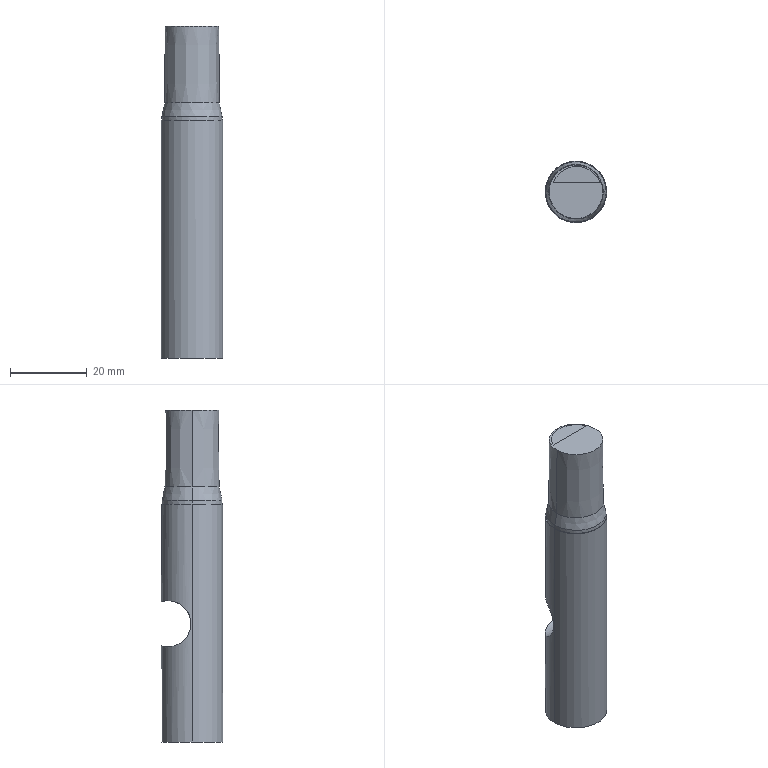Part | Creo | 1 solid | 13 faces | box 16 x 16 x 86.655 mm | volume 15519 mm3 | cylinder 5 | plane 4 | cone 4 | commonest cylinder face diameters 15.678 x2 16 x2 12 x1
STEP:
#1=CARTESIAN_POINT('',(0.,0.,0.));
#2=DIRECTION('',(0.,0.,1.));
#3=DIRECTION('',(1.,0.,0.));
#4=AXIS2_PLACEMENT_3D('',#1,#2,#3);
#5=CARTESIAN_POINT('',(-83.209,27.679,-128.582));
#6=VERTEX_POINT('',#5);
#7=CARTESIAN_POINT('',(-83.208,27.678,-116.581));
#8=VERTEX_POINT('',#7);
#9=CARTESIAN_POINT('',(-83.209,27.679,-128.582));
#10=CARTESIAN_POINT('',(-82.861,27.406,-128.582));
#11=CARTESIAN_POINT('',(-82.24,26.826,-128.543));
#12=CARTESIAN_POINT('',(-81.527,25.921,-128.344));
#13=CARTESIAN_POINT('',(-80.996,25.018,-127.988));
#14=CARTESIAN_POINT('',(-80.628,24.165,-127.48));
#15=CARTESIAN_POINT('',(-80.382,23.365,-126.798));
#16=CARTESIAN_POINT('',(-80.24,22.661,-125.935));
#17=CARTESIAN_POINT('',(-80.176,22.114,-124.925));
#18=CARTESIAN_POINT('',(-80.154,21.761,-123.789));
#19=CARTESIAN_POINT('',(-80.151,21.638,-122.589));
#20=CARTESIAN_POINT('',(-80.154,21.757,-121.388));
#21=CARTESIAN_POINT('',(-80.175,22.112,-120.237));
#22=CARTESIAN_POINT('',(-80.243,22.679,-119.196));
#23=CARTESIAN_POINT('',(-80.392,23.407,-118.321));
#24=CARTESIAN_POINT('',(-80.647,24.216,-117.646));
#25=CARTESIAN_POINT('',(-81.024,25.072,-117.148));
#26=CARTESIAN_POINT('',(-81.554,25.958,-116.808));
#27=CARTESIAN_POINT('',(-82.253,26.838,-116.618));
#28=CARTESIAN_POINT('',(-82.865,27.409,-116.581));
#29=CARTESIAN_POINT('',(-83.208,27.678,-116.581));
#30=B_SPLINE_CURVE_WITH_KNOTS('',3,(#9,#10,#11,#12,#13,#14,#15,#16,#17,#18,#19,#20,#21,#22,#23,#24,#25,#26,#27,#28,#29),.UNSPECIFIED.,.F.,.F.,(4,1,1,1,1,1,1,1,1,1,1,1,1,1,1,1,1,1,4),(0.,0.05556,0.1111,0.1667,0.2222,0.2778,0.3333,0.3889,0.4444,0.5,0.5556,0.6111,0.6667,0.7222,0.7778,0.8333,0.8889,0.9444,1.),.UNSPECIFIED.);
#31=EDGE_CURVE('',#6,#8,#30,.T.);
#32=ORIENTED_EDGE('',*,*,#31,.T.);
#33=CARTESIAN_POINT('',(-93.085,27.679,-116.581));
#34=VERTEX_POINT('',#33);
#35=CARTESIAN_POINT('',(-83.552,27.948,-116.581));
#36=CARTESIAN_POINT('',(-84.287,28.434,-116.617));
#37=CARTESIAN_POINT('',(-85.512,28.978,-116.718));
#38=CARTESIAN_POINT('',(-86.821,29.312,-116.806));
#39=CARTESIAN_POINT('',(-88.163,29.423,-116.84));
#40=CARTESIAN_POINT('',(-89.528,29.305,-116.804));
#41=CARTESIAN_POINT('',(-90.861,28.951,-116.711));
#42=CARTESIAN_POINT('',(-92.076,28.393,-116.612));
#43=CARTESIAN_POINT('',(-92.767,27.928,-116.581));
#44=CARTESIAN_POINT('',(-93.085,27.679,-116.581));
#45=B_SPLINE_CURVE_WITH_KNOTS('',3,(#7,#35,#36,#37,#38,#39,#40,#41,#42,#43,#44),.UNSPECIFIED.,.F.,.F.,(4,1,1,1,1,1,1,1,4),(0.,0.125,0.25,0.375,0.5,0.625,0.75,0.875,1.),.UNSPECIFIED.);
#46=EDGE_CURVE('',#8,#34,#45,.T.);
#47=ORIENTED_EDGE('',*,*,#46,.T.);
#48=CARTESIAN_POINT('',(-93.431,27.407,-116.581));
#49=CARTESIAN_POINT('',(-94.052,26.827,-116.618));
#50=CARTESIAN_POINT('',(-94.78,25.902,-116.823));
#51=CARTESIAN_POINT('',(-95.314,24.985,-117.189));
#52=CARTESIAN_POINT('',(-95.687,24.107,-117.721));
#53=CARTESIAN_POINT('',(-95.928,23.295,-118.435));
#54=CARTESIAN_POINT('',(-96.061,22.605,-119.313));
#55=CARTESIAN_POINT('',(-96.121,22.075,-120.331));
#56=CARTESIAN_POINT('',(-96.139,21.74,-121.477));
#57=CARTESIAN_POINT('',(-96.142,21.639,-122.684));
#58=CARTESIAN_POINT('',(-96.138,21.78,-123.88));
#59=CARTESIAN_POINT('',(-96.114,22.151,-125.013));
#60=CARTESIAN_POINT('',(-96.043,22.725,-126.032));
#61=CARTESIAN_POINT('',(-95.887,23.46,-126.895));
#62=CARTESIAN_POINT('',(-95.613,24.309,-127.584));
#63=CARTESIAN_POINT('',(-95.188,25.231,-128.091));
#64=CARTESIAN_POINT('',(-94.589,26.175,-128.416));
#65=CARTESIAN_POINT('',(-93.793,27.099,-128.576));
#66=CARTESIAN_POINT('',(-92.784,27.951,-128.592));
#67=CARTESIAN_POINT('',(-91.577,28.66,-128.511));
#68=CARTESIAN_POINT('',(-90.18,29.171,-128.397));
#69=CARTESIAN_POINT('',(-88.698,29.411,-128.326));
#70=CARTESIAN_POINT('',(-87.235,29.379,-128.336));
#71=CARTESIAN_POINT('',(-85.753,29.068,-128.424));
#72=CARTESIAN_POINT('',(-84.373,28.489,-128.539));
#73=CARTESIAN_POINT('',(-83.576,27.967,-128.582));
#74=B_SPLINE_CURVE_WITH_KNOTS('',3,(#33,#48,#49,#50,#51,#52,#53,#54,#55,#56,#57,#58,#59,#60,#61,#62,#63,#64,#65,#66,#67,#68,#69,#70,#71,#72,#73,#5),.UNSPECIFIED.,.F.,.F.,(4,1,1,1,1,1,1,1,1,1,1,1,1,1,1,1,1,1,1,1,1,1,1,1,1,4),(0.,0.04,0.08,0.12,0.16,0.2,0.24,0.28,0.32,0.36,0.4,0.44,0.48,0.52,0.56,0.6,0.64,0.68,0.72,0.76,0.8,0.84,0.88,0.92,0.96,1.),.UNSPECIFIED.);
#75=EDGE_CURVE('',#34,#6,#74,.T.);
#76=ORIENTED_EDGE('',*,*,#75,.T.);
#77=EDGE_LOOP('',(#32,#47,#76));
#78=FACE_OUTER_BOUND('',#77,.F.);
#79=CARTESIAN_POINT('',(389.101,27.678,-122.581));
#80=DIRECTION('',(-1.,0.,0.));
#81=DIRECTION('',(0.,0.,1.));
#82=AXIS2_PLACEMENT_3D('',#79,#80,#81);
#83=CYLINDRICAL_SURFACE('',#82,6.);
#84=ADVANCED_FACE('',(#78),#83,.F.);
#85=CARTESIAN_POINT('',(-96.147,21.385,-153.441));
#86=VERTEX_POINT('',#85);
#87=CARTESIAN_POINT('',(-80.147,21.385,-153.441));
#88=VERTEX_POINT('',#87);
#89=CARTESIAN_POINT('',(-88.147,21.385,-153.441));
#90=DIRECTION('',(0.,0.,-1.));
#91=DIRECTION('',(-1.,0.,0.));
#92=AXIS2_PLACEMENT_3D('',#89,#90,#91);
#93=CIRCLE('',#92,8.);
#94=EDGE_CURVE('',#86,#88,#93,.T.);
#95=ORIENTED_EDGE('',*,*,#94,.T.);
#96=CARTESIAN_POINT('',(-80.147,21.385,-91.41));
#97=VERTEX_POINT('',#96);
#98=CARTESIAN_POINT('',(-80.147,21.385,-91.41));
#99=DIRECTION('',(0.,0.,-1.));
#100=VECTOR('',#99,62.032);
#101=LINE('',#98,#100);
#102=EDGE_CURVE('',#97,#88,#101,.T.);
#103=ORIENTED_EDGE('',*,*,#102,.F.);
#104=CARTESIAN_POINT('',(-96.147,21.395,-91.389));
#105=VERTEX_POINT('',#104);
#106=CARTESIAN_POINT('',(-96.145,22.337,-91.389));
#107=CARTESIAN_POINT('',(-95.801,24.374,-91.389));
#108=CARTESIAN_POINT('',(-94.272,26.74,-91.391));
#109=CARTESIAN_POINT('',(-92.544,28.135,-91.393));
#110=CARTESIAN_POINT('',(-91.094,28.879,-91.395));
#111=CARTESIAN_POINT('',(-89.842,29.231,-91.397));
#112=CARTESIAN_POINT('',(-88.856,29.364,-91.398));
#113=CARTESIAN_POINT('',(-88.141,29.395,-91.399));
#114=CARTESIAN_POINT('',(-87.427,29.363,-91.4));
#115=CARTESIAN_POINT('',(-86.441,29.229,-91.401));
#116=CARTESIAN_POINT('',(-85.189,28.875,-91.403));
#117=CARTESIAN_POINT('',(-83.74,28.129,-91.405));
#118=CARTESIAN_POINT('',(-82.014,26.732,-91.407));
#119=CARTESIAN_POINT('',(-80.488,24.364,-91.409));
#120=CARTESIAN_POINT('',(-80.147,22.327,-91.41));
#121=B_SPLINE_CURVE_WITH_KNOTS('',3,(#104,#106,#107,#108,#109,#110,#111,#112,#113,#114,#115,#116,#117,#118,#119,#120,#96),.UNSPECIFIED.,.F.,.F.,(4,1,1,1,1,1,1,1,1,1,1,1,1,1,4),(0.,0.125,0.25,0.3125,0.375,0.4375,0.4688,0.5,0.5312,0.5625,0.625,0.6875,0.75,0.875,1.),.UNSPECIFIED.);
#122=EDGE_CURVE('',#105,#97,#121,.T.);
#123=ORIENTED_EDGE('',*,*,#122,.F.);
#124=CARTESIAN_POINT('',(-96.147,21.385,-91.389));
#125=VERTEX_POINT('',#124);
#126=CARTESIAN_POINT('',(-96.147,21.388,-91.389));
#127=CARTESIAN_POINT('',(-96.147,21.391,-91.389));
#128=CARTESIAN_POINT('',(-96.147,21.395,-91.389));
#129=B_SPLINE_CURVE_WITH_KNOTS('',3,(#124,#126,#127,#128),.UNSPECIFIED.,.F.,.F.,(4,4),(0.,1.),.UNSPECIFIED.);
#130=EDGE_CURVE('',#125,#105,#129,.T.);
#131=ORIENTED_EDGE('',*,*,#130,.F.);
#132=CARTESIAN_POINT('',(-96.147,21.385,-91.389));
#133=DIRECTION('',(-0.000000074,0.,-1.));
#134=VECTOR('',#133,62.053);
#135=LINE('',#132,#134);
#136=EDGE_CURVE('',#125,#86,#135,.T.);
#137=ORIENTED_EDGE('',*,*,#136,.T.);
#138=EDGE_LOOP('',(#95,#103,#123,#131,#137));
#139=FACE_OUTER_BOUND('',#138,.F.);
#140=ORIENTED_EDGE('',*,*,#75,.F.);
#141=ORIENTED_EDGE('',*,*,#46,.F.);
#142=ORIENTED_EDGE('',*,*,#31,.F.);
#143=EDGE_LOOP('',(#140,#141,#142));
#144=FACE_BOUND('',#143,.F.);
#145=CARTESIAN_POINT('',(-88.147,21.385,508.193));
#146=DIRECTION('',(0.,0.,-1.));
#147=DIRECTION('',(-1.,0.,0.));
#148=AXIS2_PLACEMENT_3D('',#145,#146,#147);
#149=CYLINDRICAL_SURFACE('',#148,8.);
#150=ADVANCED_FACE('',(#139,#144),#149,.T.);
#151=ORIENTED_EDGE('',*,*,#94,.F.);
#152=CARTESIAN_POINT('',(-88.147,21.385,-153.441));
#153=DIRECTION('',(0.,0.,-1.));
#154=DIRECTION('',(1.,0.,0.));
#155=AXIS2_PLACEMENT_3D('',#152,#153,#154);
#156=CIRCLE('',#155,8.);
#157=EDGE_CURVE('',#88,#86,#156,.T.);
#158=ORIENTED_EDGE('',*,*,#157,.F.);
#159=EDGE_LOOP('',(#151,#158));
#160=FACE_OUTER_BOUND('',#159,.F.);
#161=CARTESIAN_POINT('',(5.725,319.968,-153.441));
#162=DIRECTION('',(0.,0.,-1.));
#163=DIRECTION('',(-1.,0.,0.));
#164=AXIS2_PLACEMENT_3D('',#161,#162,#163);
#165=PLANE('',#164);
#166=ADVANCED_FACE('',(#160),#165,.T.);
#167=ORIENTED_EDGE('',*,*,#157,.T.);
#168=ORIENTED_EDGE('',*,*,#136,.F.);
#169=CARTESIAN_POINT('',(-80.147,21.375,-91.41));
#170=VERTEX_POINT('',#169);
#171=CARTESIAN_POINT('',(-80.147,20.879,-91.41));
#172=CARTESIAN_POINT('',(-80.239,19.905,-91.41));
#173=CARTESIAN_POINT('',(-80.645,18.475,-91.409));
#174=CARTESIAN_POINT('',(-81.31,17.144,-91.408));
#175=CARTESIAN_POINT('',(-82.196,15.97,-91.407));
#176=CARTESIAN_POINT('',(-83.297,14.964,-91.406));
#177=CARTESIAN_POINT('',(-84.565,14.18,-91.404));
#178=CARTESIAN_POINT('',(-85.953,13.644,-91.402));
#179=CARTESIAN_POINT('',(-87.413,13.373,-91.4));
#180=CARTESIAN_POINT('',(-88.896,13.374,-91.398));
#181=CARTESIAN_POINT('',(-90.351,13.647,-91.396));
#182=CARTESIAN_POINT('',(-91.732,14.183,-91.395));
#183=CARTESIAN_POINT('',(-92.993,14.962,-91.393));
#184=CARTESIAN_POINT('',(-94.092,15.964,-91.391));
#185=CARTESIAN_POINT('',(-94.979,17.137,-91.39));
#186=CARTESIAN_POINT('',(-95.647,18.47,-91.389));
#187=CARTESIAN_POINT('',(-96.055,19.907,-91.389));
#188=CARTESIAN_POINT('',(-96.147,20.886,-91.389));
#189=CARTESIAN_POINT('',(-96.147,21.385,-91.389));
#190=B_SPLINE_CURVE_WITH_KNOTS('',3,(#169,#171,#172,#173,#174,#175,#176,#177,#178,#179,#180,#181,#182,#183,#184,#185,#186,#187,#188,#189),.UNSPECIFIED.,.F.,.F.,(4,1,1,1,1,1,1,1,1,1,1,1,1,1,1,1,1,4),(0.,0.05882,0.1176,0.1765,0.2353,0.2941,0.3529,0.4118,0.4706,0.5294,0.5882,0.6471,0.7059,0.7647,0.8235,0.8824,0.9412,1.),.UNSPECIFIED.);
#191=EDGE_CURVE('',#170,#125,#190,.T.);
#192=ORIENTED_EDGE('',*,*,#191,.F.);
#193=CARTESIAN_POINT('',(-80.147,21.385,-91.41));
#194=CARTESIAN_POINT('',(-80.147,21.381,-91.41));
#195=CARTESIAN_POINT('',(-80.147,21.378,-91.41));
#196=CARTESIAN_POINT('',(-80.147,21.375,-91.41));
#197=B_SPLINE_CURVE_WITH_KNOTS('',3,(#193,#194,#195,#196),.UNSPECIFIED.,.F.,.F.,(4,4),(0.,1.),.UNSPECIFIED.);
#198=EDGE_CURVE('',#97,#170,#197,.T.);
#199=ORIENTED_EDGE('',*,*,#198,.F.);
#200=ORIENTED_EDGE('',*,*,#102,.T.);
#201=EDGE_LOOP('',(#167,#168,#192,#199,#200));
#202=FACE_OUTER_BOUND('',#201,.F.);
#203=CARTESIAN_POINT('',(-88.147,21.385,508.193));
#204=DIRECTION('',(0.,0.,-1.));
#205=DIRECTION('',(-1.,0.,0.));
#206=AXIS2_PLACEMENT_3D('',#203,#204,#205);
#207=CYLINDRICAL_SURFACE('',#206,8.);
#208=ADVANCED_FACE('',(#202),#207,.T.);
#209=ORIENTED_EDGE('',*,*,#191,.T.);
#210=ORIENTED_EDGE('',*,*,#130,.T.);
#211=ORIENTED_EDGE('',*,*,#122,.T.);
#212=ORIENTED_EDGE('',*,*,#198,.T.);
#213=EDGE_LOOP('',(#209,#210,#211,#212));
#214=FACE_OUTER_BOUND('',#213,.F.);
#215=CARTESIAN_POINT('',(-80.308,21.375,-91.41));
#216=VERTEX_POINT('',#215);
#217=CARTESIAN_POINT('',(-80.308,21.385,-91.41));
#218=VERTEX_POINT('',#217);
#219=CARTESIAN_POINT('',(-80.308,21.378,-91.41));
#220=CARTESIAN_POINT('',(-80.308,21.381,-91.41));
#221=CARTESIAN_POINT('',(-80.308,21.385,-91.41));
#222=B_SPLINE_CURVE_WITH_KNOTS('',3,(#215,#219,#220,#221),.UNSPECIFIED.,.F.,.F.,(4,4),(0.,1.),.UNSPECIFIED.);
#223=EDGE_CURVE('',#216,#218,#222,.T.);
#224=ORIENTED_EDGE('',*,*,#223,.T.);
#225=CARTESIAN_POINT('',(-95.986,21.395,-91.389));
#226=VERTEX_POINT('',#225);
#227=CARTESIAN_POINT('',(-80.308,21.87,-91.41));
#228=CARTESIAN_POINT('',(-80.396,22.825,-91.409));
#229=CARTESIAN_POINT('',(-80.792,24.227,-91.409));
#230=CARTESIAN_POINT('',(-81.442,25.532,-91.408));
#231=CARTESIAN_POINT('',(-82.309,26.683,-91.407));
#232=CARTESIAN_POINT('',(-83.386,27.67,-91.405));
#233=CARTESIAN_POINT('',(-84.627,28.44,-91.404));
#234=CARTESIAN_POINT('',(-85.987,28.967,-91.402));
#235=CARTESIAN_POINT('',(-87.417,29.235,-91.4));
#236=CARTESIAN_POINT('',(-88.87,29.235,-91.398));
#237=CARTESIAN_POINT('',(-90.297,28.969,-91.396));
#238=CARTESIAN_POINT('',(-91.651,28.447,-91.395));
#239=CARTESIAN_POINT('',(-92.887,27.684,-91.393));
#240=CARTESIAN_POINT('',(-93.965,26.704,-91.392));
#241=CARTESIAN_POINT('',(-94.836,25.556,-91.39));
#242=CARTESIAN_POINT('',(-95.492,24.25,-91.39));
#243=CARTESIAN_POINT('',(-95.894,22.842,-91.389));
#244=CARTESIAN_POINT('',(-95.985,21.883,-91.389));
#245=CARTESIAN_POINT('',(-95.986,21.395,-91.389));
#246=B_SPLINE_CURVE_WITH_KNOTS('',3,(#217,#227,#228,#229,#230,#231,#232,#233,#234,#235,#236,#237,#238,#239,#240,#241,#242,#243,#244,#245),.UNSPECIFIED.,.F.,.F.,(4,1,1,1,1,1,1,1,1,1,1,1,1,1,1,1,1,4),(0.,0.05882,0.1176,0.1765,0.2353,0.2941,0.3529,0.4118,0.4706,0.5294,0.5882,0.6471,0.7059,0.7647,0.8235,0.8824,0.9412,1.),.UNSPECIFIED.);
#247=EDGE_CURVE('',#218,#226,#246,.T.);
#248=ORIENTED_EDGE('',*,*,#247,.T.);
#249=CARTESIAN_POINT('',(-95.986,21.385,-91.389));
#250=VERTEX_POINT('',#249);
#251=CARTESIAN_POINT('',(-95.986,21.391,-91.389));
#252=CARTESIAN_POINT('',(-95.986,21.388,-91.389));
#253=B_SPLINE_CURVE_WITH_KNOTS('',3,(#225,#251,#252,#249),.UNSPECIFIED.,.F.,.F.,(4,4),(0.,1.),.UNSPECIFIED.);
#254=EDGE_CURVE('',#226,#250,#253,.T.);
#255=ORIENTED_EDGE('',*,*,#254,.T.);
#256=CARTESIAN_POINT('',(-95.986,21.385,-91.389));
#257=CARTESIAN_POINT('',(-95.986,20.461,-91.389));
#258=CARTESIAN_POINT('',(-95.651,18.465,-91.389));
#259=CARTESIAN_POINT('',(-94.155,16.145,-91.391));
#260=CARTESIAN_POINT('',(-92.464,14.776,-91.394));
#261=CARTESIAN_POINT('',(-91.044,14.045,-91.395));
#262=CARTESIAN_POINT('',(-89.818,13.698,-91.397));
#263=CARTESIAN_POINT('',(-88.852,13.567,-91.398));
#264=CARTESIAN_POINT('',(-88.152,13.535,-91.399));
#265=CARTESIAN_POINT('',(-87.451,13.566,-91.4));
#266=CARTESIAN_POINT('',(-86.485,13.696,-91.401));
#267=CARTESIAN_POINT('',(-85.258,14.041,-91.403));
#268=CARTESIAN_POINT('',(-83.837,14.77,-91.405));
#269=CARTESIAN_POINT('',(-82.144,16.138,-91.407));
#270=CARTESIAN_POINT('',(-80.646,18.456,-91.409));
#271=CARTESIAN_POINT('',(-80.309,20.451,-91.41));
#272=CARTESIAN_POINT('',(-80.308,21.375,-91.41));
#273=B_SPLINE_CURVE_WITH_KNOTS('',3,(#256,#257,#258,#259,#260,#261,#262,#263,#264,#265,#266,#267,#268,#269,#270,#271,#272),.UNSPECIFIED.,.F.,.F.,(4,1,1,1,1,1,1,1,1,1,1,1,1,1,4),(0.,0.125,0.25,0.3125,0.375,0.4375,0.4688,0.5,0.5312,0.5625,0.625,0.6875,0.75,0.875,1.),.UNSPECIFIED.);
#274=EDGE_CURVE('',#250,#216,#273,.T.);
#275=ORIENTED_EDGE('',*,*,#274,.T.);
#276=EDGE_LOOP('',(#224,#248,#255,#275));
#277=FACE_BOUND('',#276,.F.);
#278=CARTESIAN_POINT('',(248.993,54.022,-91.842));
#279=DIRECTION('',(-0.001312,0.000001665,-1.));
#280=DIRECTION('',(-1.,0.,0.001312));
#281=AXIS2_PLACEMENT_3D('',#278,#279,#280);
#282=PLANE('',#281);
#283=ADVANCED_FACE('',(#214,#277),#282,.F.);
#284=CARTESIAN_POINT('',(-95.987,21.385,-90.394));
#285=VERTEX_POINT('',#284);
#286=CARTESIAN_POINT('',(-80.307,21.385,-90.394));
#287=VERTEX_POINT('',#286);
#288=CARTESIAN_POINT('',(-88.148,21.385,-90.394));
#289=DIRECTION('',(0.00002709,0.,1.));
#290=DIRECTION('',(-1.,0.,0.00002709));
#291=AXIS2_PLACEMENT_3D('',#288,#289,#290);
#292=CIRCLE('',#291,7.841);
#293=EDGE_CURVE('',#285,#287,#292,.T.);
#294=ORIENTED_EDGE('',*,*,#293,.T.);
#295=CARTESIAN_POINT('',(-80.308,21.385,-91.41));
#296=DIRECTION('',(0.0003927,0.000000008,1.));
#297=VECTOR('',#296,1.015);
#298=LINE('',#295,#297);
#299=EDGE_CURVE('',#218,#287,#298,.T.);
#300=ORIENTED_EDGE('',*,*,#299,.F.);
#301=ORIENTED_EDGE('',*,*,#223,.F.);
#302=ORIENTED_EDGE('',*,*,#274,.F.);
#303=CARTESIAN_POINT('',(-95.986,21.385,-91.389));
#304=DIRECTION('',(-0.001462,0.,1.));
#305=VECTOR('',#304,0.995);
#306=LINE('',#303,#305);
#307=EDGE_CURVE('',#250,#285,#306,.T.);
#308=ORIENTED_EDGE('',*,*,#307,.T.);
#309=EDGE_LOOP('',(#294,#300,#301,#302,#308));
#310=FACE_OUTER_BOUND('',#309,.F.);
#311=CARTESIAN_POINT('',(-88.147,21.385,-91.399));
#312=DIRECTION('',(0.,0.,1.));
#313=DIRECTION('',(1.,0.,0.));
#314=AXIS2_PLACEMENT_3D('',#311,#312,#313);
#315=CYLINDRICAL_SURFACE('',#314,7.839);
#316=ADVANCED_FACE('',(#310),#315,.T.);
#317=CARTESIAN_POINT('',(-95.283,21.385,-86.876));
#318=VERTEX_POINT('',#317);
#319=CARTESIAN_POINT('',(-81.011,21.385,-86.877));
#320=VERTEX_POINT('',#319);
#321=CARTESIAN_POINT('',(-88.147,21.385,-86.877));
#322=DIRECTION('',(0.,0.,1.));
#323=DIRECTION('',(-1.,0.,0.));
#324=AXIS2_PLACEMENT_3D('',#321,#322,#323);
#325=CIRCLE('',#324,7.136);
#326=EDGE_CURVE('',#318,#320,#325,.T.);
#327=ORIENTED_EDGE('',*,*,#326,.T.);
#328=CARTESIAN_POINT('',(-81.011,21.385,-86.877));
#329=DIRECTION('',(0.1961,0.,-0.9806));
#330=VECTOR('',#329,3.587);
#331=LINE('',#328,#330);
#332=EDGE_CURVE('',#320,#287,#331,.T.);
#333=ORIENTED_EDGE('',*,*,#332,.T.);
#334=ORIENTED_EDGE('',*,*,#293,.F.);
#335=CARTESIAN_POINT('',(-95.283,21.385,-86.876));
#336=DIRECTION('',(-0.1962,0.,-0.9806));
#337=VECTOR('',#336,3.587);
#338=LINE('',#335,#337);
#339=EDGE_CURVE('',#318,#285,#338,.T.);
#340=ORIENTED_EDGE('',*,*,#339,.F.);
#341=EDGE_LOOP('',(#327,#333,#334,#340));
#342=FACE_OUTER_BOUND('',#341,.F.);
#343=CARTESIAN_POINT('',(-88.148,21.385,-88.635));
#344=DIRECTION('',(-0.00002709,0.,-1.));
#345=DIRECTION('',(1.,0.,-0.00002709));
#346=AXIS2_PLACEMENT_3D('',#343,#344,#345);
#347=CONICAL_SURFACE('',#346,7.489,11.313);
#348=ADVANCED_FACE('',(#342),#347,.T.);
#349=ORIENTED_EDGE('',*,*,#326,.F.);
#350=CARTESIAN_POINT('',(-95.142,21.385,-66.85));
#351=VERTEX_POINT('',#350);
#352=CARTESIAN_POINT('',(-95.142,21.385,-66.85));
#353=DIRECTION('',(-0.007048,0.,-1.));
#354=VECTOR('',#353,20.027);
#355=LINE('',#352,#354);
#356=EDGE_CURVE('',#351,#318,#355,.T.);
#357=ORIENTED_EDGE('',*,*,#356,.F.);
#358=CARTESIAN_POINT('',(-81.151,21.385,-66.868));
#359=VERTEX_POINT('',#358);
#360=CARTESIAN_POINT('',(-95.142,21.385,-66.85));
#361=CARTESIAN_POINT('',(-95.142,20.56,-66.841));
#362=CARTESIAN_POINT('',(-94.843,18.778,-66.823));
#363=CARTESIAN_POINT('',(-93.508,16.708,-66.804));
#364=CARTESIAN_POINT('',(-91.997,15.486,-66.793));
#365=CARTESIAN_POINT('',(-90.731,14.834,-66.788));
#366=CARTESIAN_POINT('',(-89.41,14.463,-66.786));
#367=CARTESIAN_POINT('',(-88.146,14.353,-66.786));
#368=CARTESIAN_POINT('',(-86.883,14.463,-66.789));
#369=CARTESIAN_POINT('',(-85.562,14.834,-66.795));
#370=CARTESIAN_POINT('',(-84.296,15.486,-66.803));
#371=CARTESIAN_POINT('',(-82.785,16.708,-66.818));
#372=CARTESIAN_POINT('',(-81.45,18.778,-66.841));
#373=CARTESIAN_POINT('',(-81.151,20.56,-66.859));
#374=CARTESIAN_POINT('',(-81.151,21.385,-66.868));
#375=B_SPLINE_CURVE_WITH_KNOTS('',3,(#360,#361,#362,#363,#364,#365,#366,#367,#368,#369,#370,#371,#372,#373,#374),.UNSPECIFIED.,.F.,.F.,(4,1,1,1,1,1,1,1,1,1,1,1,4),(0.,0.125,0.25,0.3125,0.375,0.4375,0.5,0.5625,0.625,0.6875,0.75,0.875,1.),.UNSPECIFIED.);
#376=EDGE_CURVE('',#351,#359,#375,.T.);
#377=ORIENTED_EDGE('',*,*,#376,.T.);
#378=CARTESIAN_POINT('',(-81.151,21.385,-66.868));
#379=DIRECTION('',(0.007,0.,-1.));
#380=VECTOR('',#379,20.009);
#381=LINE('',#378,#380);
#382=EDGE_CURVE('',#359,#320,#381,.T.);
#383=ORIENTED_EDGE('',*,*,#382,.T.);
#384=EDGE_LOOP('',(#349,#357,#377,#383));
#385=FACE_OUTER_BOUND('',#384,.F.);
#386=CARTESIAN_POINT('',(-88.147,21.385,-76.831));
#387=DIRECTION('',(0.,0.,-1.));
#388=DIRECTION('',(1.,0.,0.));
#389=AXIS2_PLACEMENT_3D('',#386,#387,#388);
#390=CONICAL_SURFACE('',#389,7.065,0.4);
#391=ADVANCED_FACE('',(#385),#390,.T.);
#392=CARTESIAN_POINT('',(-88.147,21.385,-86.877));
#393=DIRECTION('',(0.,0.,1.));
#394=DIRECTION('',(1.,0.,0.));
#395=AXIS2_PLACEMENT_3D('',#392,#393,#394);
#396=CIRCLE('',#395,7.136);
#397=EDGE_CURVE('',#320,#318,#396,.T.);
#398=ORIENTED_EDGE('',*,*,#397,.F.);
#399=ORIENTED_EDGE('',*,*,#382,.F.);
#400=CARTESIAN_POINT('',(-87.267,28.325,-66.931));
#401=VERTEX_POINT('',#400);
#402=CARTESIAN_POINT('',(-81.151,21.385,-66.868));
#403=CARTESIAN_POINT('',(-81.151,21.898,-66.873));
#404=CARTESIAN_POINT('',(-81.259,22.83,-66.883));
#405=CARTESIAN_POINT('',(-81.762,24.443,-66.899));
#406=CARTESIAN_POINT('',(-82.806,26.091,-66.914));
#407=CARTESIAN_POINT('',(-84.31,27.335,-66.925));
#408=CARTESIAN_POINT('',(-85.847,28.036,-66.93));
#409=CARTESIAN_POINT('',(-86.757,28.261,-66.931));
#410=B_SPLINE_CURVE_WITH_KNOTS('',3,(#402,#403,#404,#405,#406,#407,#408,#409,#400),.UNSPECIFIED.,.F.,.F.,(4,1,1,1,1,1,4),(0.,0.125,0.25,0.5,0.75,0.875,1.),.UNSPECIFIED.);
#411=EDGE_CURVE('',#359,#401,#410,.T.);
#412=ORIENTED_EDGE('',*,*,#411,.T.);
#413=CARTESIAN_POINT('',(-87.267,28.325,-66.931));
#414=CARTESIAN_POINT('',(-87.923,28.409,-66.931));
#415=CARTESIAN_POINT('',(-89.062,28.378,-66.93));
#416=CARTESIAN_POINT('',(-90.977,27.905,-66.922));
#417=CARTESIAN_POINT('',(-92.875,26.75,-66.908));
#418=CARTESIAN_POINT('',(-94.258,25.013,-66.888));
#419=CARTESIAN_POINT('',(-94.969,23.173,-66.868));
#420=CARTESIAN_POINT('',(-95.142,22.046,-66.856));
#421=CARTESIAN_POINT('',(-95.142,21.385,-66.85));
#422=B_SPLINE_CURVE_WITH_KNOTS('',3,(#413,#414,#415,#416,#417,#418,#419,#420,#421),.UNSPECIFIED.,.F.,.F.,(4,1,1,1,1,1,4),(0.,0.125,0.25,0.5,0.75,0.875,1.),.UNSPECIFIED.);
#423=EDGE_CURVE('',#401,#351,#422,.T.);
#424=ORIENTED_EDGE('',*,*,#423,.T.);
#425=ORIENTED_EDGE('',*,*,#356,.T.);
#426=EDGE_LOOP('',(#398,#399,#412,#424,#425));
#427=FACE_OUTER_BOUND('',#426,.F.);
#428=CARTESIAN_POINT('',(-88.147,21.385,-76.863));
#429=DIRECTION('',(0.,0.,-1.));
#430=DIRECTION('',(1.,0.,0.));
#431=AXIS2_PLACEMENT_3D('',#428,#429,#430);
#432=CONICAL_SURFACE('',#431,7.066,0.4);
#433=ADVANCED_FACE('',(#427),#432,.T.);
#434=ORIENTED_EDGE('',*,*,#397,.T.);
#435=ORIENTED_EDGE('',*,*,#339,.T.);
#436=CARTESIAN_POINT('',(-88.148,21.385,-90.394));
#437=DIRECTION('',(0.00002709,0.,1.));
#438=DIRECTION('',(1.,0.,-0.00002709));
#439=AXIS2_PLACEMENT_3D('',#436,#437,#438);
#440=CIRCLE('',#439,7.841);
#441=EDGE_CURVE('',#287,#285,#440,.T.);
#442=ORIENTED_EDGE('',*,*,#441,.F.);
#443=ORIENTED_EDGE('',*,*,#332,.F.);
#444=EDGE_LOOP('',(#434,#435,#442,#443));
#445=FACE_OUTER_BOUND('',#444,.F.);
#446=CARTESIAN_POINT('',(-88.148,21.385,-88.635));
#447=DIRECTION('',(-0.00002709,0.,-1.));
#448=DIRECTION('',(1.,0.,-0.00002709));
#449=AXIS2_PLACEMENT_3D('',#446,#447,#448);
#450=CONICAL_SURFACE('',#449,7.489,11.313);
#451=ADVANCED_FACE('',(#445),#450,.T.);
#452=ORIENTED_EDGE('',*,*,#441,.T.);
#453=ORIENTED_EDGE('',*,*,#307,.F.);
#454=ORIENTED_EDGE('',*,*,#254,.F.);
#455=ORIENTED_EDGE('',*,*,#247,.F.);
#456=ORIENTED_EDGE('',*,*,#299,.T.);
#457=EDGE_LOOP('',(#452,#453,#454,#455,#456));
#458=FACE_OUTER_BOUND('',#457,.F.);
#459=CARTESIAN_POINT('',(-88.147,21.385,-91.399));
#460=DIRECTION('',(0.,0.,1.));
#461=DIRECTION('',(1.,0.,0.));
#462=AXIS2_PLACEMENT_3D('',#459,#460,#461);
#463=CYLINDRICAL_SURFACE('',#462,7.839);
#464=ADVANCED_FACE('',(#458),#463,.T.);
#465=ORIENTED_EDGE('',*,*,#423,.F.);
#466=ORIENTED_EDGE('',*,*,#411,.F.);
#467=ORIENTED_EDGE('',*,*,#376,.F.);
#468=EDGE_LOOP('',(#465,#466,#467));
#469=FACE_OUTER_BOUND('',#468,.F.);
#470=CARTESIAN_POINT('',(-94.13,23.766,-66.875));
#471=VERTEX_POINT('',#470);
#472=CARTESIAN_POINT('',(-81.799,23.766,-66.892));
#473=VERTEX_POINT('',#472);
#474=CARTESIAN_POINT('',(-94.13,23.766,-66.875));
#475=CARTESIAN_POINT('',(-93.967,24.184,-66.88));
#476=CARTESIAN_POINT('',(-93.57,24.97,-66.889));
#477=CARTESIAN_POINT('',(-92.741,26.018,-66.9));
#478=CARTESIAN_POINT('',(-91.724,26.875,-66.911));
#479=CARTESIAN_POINT('',(-90.557,27.513,-66.919));
#480=CARTESIAN_POINT('',(-89.287,27.906,-66.924));
#481=CARTESIAN_POINT('',(-87.965,28.039,-66.927));
#482=CARTESIAN_POINT('',(-86.643,27.906,-66.928));
#483=CARTESIAN_POINT('',(-85.373,27.513,-66.925));
#484=CARTESIAN_POINT('',(-84.206,26.875,-66.92));
#485=CARTESIAN_POINT('',(-83.189,26.018,-66.913));
#486=CARTESIAN_POINT('',(-82.36,24.97,-66.903));
#487=CARTESIAN_POINT('',(-81.962,24.184,-66.896));
#488=CARTESIAN_POINT('',(-81.799,23.766,-66.892));
#489=B_SPLINE_CURVE_WITH_KNOTS('',3,(#474,#475,#476,#477,#478,#479,#480,#481,#482,#483,#484,#485,#486,#487,#488),.UNSPECIFIED.,.F.,.F.,(4,1,1,1,1,1,1,1,1,1,1,1,4),(0.,0.08333,0.1667,0.25,0.3333,0.4167,0.5,0.5833,0.6667,0.75,0.8333,0.9167,1.),.UNSPECIFIED.);
#490=EDGE_CURVE('',#471,#473,#489,.T.);
#491=ORIENTED_EDGE('',*,*,#490,.F.);
#492=CARTESIAN_POINT('',(-81.799,23.766,-66.892));
#493=DIRECTION('',(-1.,-0.000008505,0.001305));
#494=VECTOR('',#493,12.33);
#495=LINE('',#492,#494);
#496=EDGE_CURVE('',#473,#471,#495,.T.);
#497=ORIENTED_EDGE('',*,*,#496,.F.);
#498=EDGE_LOOP('',(#491,#497));
#499=FACE_BOUND('',#498,.F.);
#500=CARTESIAN_POINT('',(-107.227,32.035,-66.944));
#501=DIRECTION('',(-0.001305,-0.0103,-0.9999));
#502=DIRECTION('',(0.,0.9999,-0.0103));
#503=AXIS2_PLACEMENT_3D('',#500,#501,#502);
#504=PLANE('',#503);
#505=ADVANCED_FACE('',(#469,#499),#504,.F.);
#506=ORIENTED_EDGE('',*,*,#496,.T.);
#507=ORIENTED_EDGE('',*,*,#490,.T.);
#508=EDGE_LOOP('',(#506,#507));
#509=FACE_OUTER_BOUND('',#508,.F.);
#510=CARTESIAN_POINT('',(-107.227,32.035,-66.944));
#511=DIRECTION('',(-0.001305,-0.0103,-0.9999));
#512=DIRECTION('',(0.,0.9999,-0.0103));
#513=AXIS2_PLACEMENT_3D('',#510,#511,#512);
#514=PLANE('',#513);
#515=ADVANCED_FACE('',(#509),#514,.F.);
#516=CLOSED_SHELL('',(#84,#150,#166,#208,#283,#316,#348,#391,#433,#451,#464,#505,#515));
#517=MANIFOLD_SOLID_BREP('',#516);
#518=(LENGTH_UNIT()NAMED_UNIT(*)SI_UNIT(.MILLI.,.METRE.));
#519=UNCERTAINTY_MEASURE_WITH_UNIT(LENGTH_MEASURE(0.008957),#518,'','');
#520=(NAMED_UNIT(*)PLANE_ANGLE_UNIT()SI_UNIT($,.RADIAN.));
#521=PLANE_ANGLE_MEASURE_WITH_UNIT(PLANE_ANGLE_MEASURE(0.01745),#520);
#522=(CONVERSION_BASED_UNIT('DEGREE',#521)NAMED_UNIT(*)PLANE_ANGLE_UNIT());
#523=(NAMED_UNIT(*)SI_UNIT($,.STERADIAN.)SOLID_ANGLE_UNIT());
#524=(GEOMETRIC_REPRESENTATION_CONTEXT(3)GLOBAL_UNCERTAINTY_ASSIGNED_CONTEXT((#519))GLOBAL_UNIT_ASSIGNED_CONTEXT((#518,#522,#523))REPRESENTATION_CONTEXT('',''));
#525=ADVANCED_BREP_SHAPE_REPRESENTATION('',(#4,#517),#524);